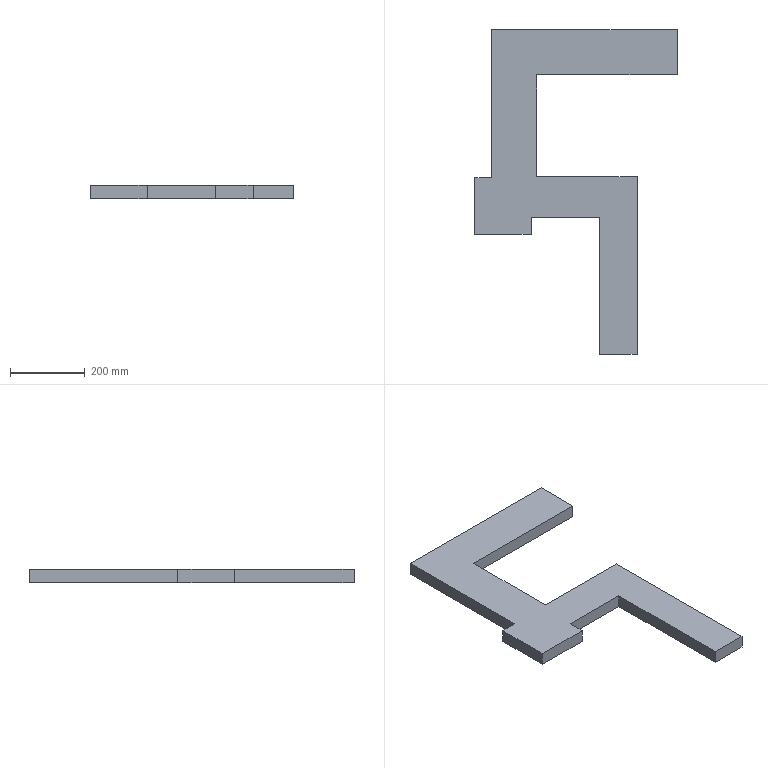Part | SolidWorks | features Extrusion 1 | 1 solid | 16 faces | box 540 x 865 x 35 mm | volume 6369754 mm3 | plane 16
STEP:
#1=CARTESIAN_POINT('',(0.,-120.,0.));
#2=VERTEX_POINT('',#1);
#3=CARTESIAN_POINT('',(0.,0.,0.));
#4=VERTEX_POINT('',#3);
#5=CARTESIAN_POINT('',(0.,0.,0.));
#6=DIRECTION('',(0.,1.,0.));
#7=VECTOR('',#6,1000.);
#8=LINE('',#5,#7);
#9=EDGE_CURVE('',#2,#4,#8,.T.);
#10=ORIENTED_EDGE('',*,*,#9,.T.);
#11=CARTESIAN_POINT('',(0.,0.,35.));
#12=VERTEX_POINT('',#11);
#13=CARTESIAN_POINT('',(0.,0.,35.));
#14=DIRECTION('',(0.,0.,-1.));
#15=VECTOR('',#14,1000.);
#16=LINE('',#13,#15);
#17=EDGE_CURVE('',#12,#4,#16,.T.);
#18=ORIENTED_EDGE('',*,*,#17,.F.);
#19=CARTESIAN_POINT('',(0.,-120.,35.));
#20=VERTEX_POINT('',#19);
#21=CARTESIAN_POINT('',(0.,0.,35.));
#22=DIRECTION('',(0.,1.,0.));
#23=VECTOR('',#22,1000.);
#24=LINE('',#21,#23);
#25=EDGE_CURVE('',#20,#12,#24,.T.);
#26=ORIENTED_EDGE('',*,*,#25,.F.);
#27=CARTESIAN_POINT('',(0.,-120.,35.));
#28=DIRECTION('',(0.,0.,-1.));
#29=VECTOR('',#28,1000.);
#30=LINE('',#27,#29);
#31=EDGE_CURVE('',#20,#2,#30,.T.);
#32=ORIENTED_EDGE('',*,*,#31,.T.);
#33=EDGE_LOOP('',(#10,#18,#26,#32));
#34=FACE_OUTER_BOUND('',#33,.T.);
#35=CARTESIAN_POINT('',(0.,0.,35.));
#36=DIRECTION('',(-1.,0.,0.));
#37=DIRECTION('',(0.,0.,1.));
#38=AXIS2_PLACEMENT_3D('',#35,#36,#37);
#39=PLANE('',#38);
#40=ADVANCED_FACE('',(#34),#39,.F.);
#41=CARTESIAN_POINT('',(-495.,0.,0.));
#42=VERTEX_POINT('',#41);
#43=CARTESIAN_POINT('',(0.,0.,0.));
#44=DIRECTION('',(-1.,0.,0.));
#45=VECTOR('',#44,1000.);
#46=LINE('',#43,#45);
#47=EDGE_CURVE('',#4,#42,#46,.T.);
#48=ORIENTED_EDGE('',*,*,#47,.T.);
#49=CARTESIAN_POINT('',(-495.,0.,35.));
#50=VERTEX_POINT('',#49);
#51=CARTESIAN_POINT('',(-495.,0.,35.));
#52=DIRECTION('',(0.,0.,-1.));
#53=VECTOR('',#52,1000.);
#54=LINE('',#51,#53);
#55=EDGE_CURVE('',#50,#42,#54,.T.);
#56=ORIENTED_EDGE('',*,*,#55,.F.);
#57=CARTESIAN_POINT('',(0.,0.,35.));
#58=DIRECTION('',(-1.,0.,0.));
#59=VECTOR('',#58,1000.);
#60=LINE('',#57,#59);
#61=EDGE_CURVE('',#12,#50,#60,.T.);
#62=ORIENTED_EDGE('',*,*,#61,.F.);
#63=ORIENTED_EDGE('',*,*,#17,.T.);
#64=EDGE_LOOP('',(#48,#56,#62,#63));
#65=FACE_OUTER_BOUND('',#64,.T.);
#66=CARTESIAN_POINT('',(0.,0.,35.));
#67=DIRECTION('',(0.,-1.,0.));
#68=DIRECTION('',(1.,0.,0.));
#69=AXIS2_PLACEMENT_3D('',#66,#67,#68);
#70=PLANE('',#69);
#71=ADVANCED_FACE('',(#65),#70,.F.);
#72=CARTESIAN_POINT('',(-495.,-395.,0.));
#73=VERTEX_POINT('',#72);
#74=CARTESIAN_POINT('',(-495.,-395.,0.));
#75=DIRECTION('',(0.,-1.,0.));
#76=VECTOR('',#75,1000.);
#77=LINE('',#74,#76);
#78=EDGE_CURVE('',#42,#73,#77,.T.);
#79=ORIENTED_EDGE('',*,*,#78,.T.);
#80=CARTESIAN_POINT('',(-495.,-395.,35.));
#81=VERTEX_POINT('',#80);
#82=CARTESIAN_POINT('',(-495.,-395.,35.));
#83=DIRECTION('',(0.,0.,-1.));
#84=VECTOR('',#83,1000.);
#85=LINE('',#82,#84);
#86=EDGE_CURVE('',#81,#73,#85,.T.);
#87=ORIENTED_EDGE('',*,*,#86,.F.);
#88=CARTESIAN_POINT('',(-495.,-395.,35.));
#89=DIRECTION('',(0.,-1.,0.));
#90=VECTOR('',#89,1000.);
#91=LINE('',#88,#90);
#92=EDGE_CURVE('',#50,#81,#91,.T.);
#93=ORIENTED_EDGE('',*,*,#92,.F.);
#94=ORIENTED_EDGE('',*,*,#55,.T.);
#95=EDGE_LOOP('',(#79,#87,#93,#94));
#96=FACE_OUTER_BOUND('',#95,.T.);
#97=CARTESIAN_POINT('',(-495.,-395.,35.));
#98=DIRECTION('',(1.,0.,0.));
#99=DIRECTION('',(0.,0.,-1.));
#100=AXIS2_PLACEMENT_3D('',#97,#98,#99);
#101=PLANE('',#100);
#102=ADVANCED_FACE('',(#96),#101,.F.);
#103=CARTESIAN_POINT('',(-540.,-395.,0.));
#104=VERTEX_POINT('',#103);
#105=CARTESIAN_POINT('',(-495.,-395.,0.));
#106=DIRECTION('',(-1.,0.,0.));
#107=VECTOR('',#106,1000.);
#108=LINE('',#105,#107);
#109=EDGE_CURVE('',#73,#104,#108,.T.);
#110=ORIENTED_EDGE('',*,*,#109,.T.);
#111=CARTESIAN_POINT('',(-540.,-395.,35.));
#112=VERTEX_POINT('',#111);
#113=CARTESIAN_POINT('',(-540.,-395.,35.));
#114=DIRECTION('',(0.,0.,-1.));
#115=VECTOR('',#114,1000.);
#116=LINE('',#113,#115);
#117=EDGE_CURVE('',#112,#104,#116,.T.);
#118=ORIENTED_EDGE('',*,*,#117,.F.);
#119=CARTESIAN_POINT('',(-495.,-395.,35.));
#120=DIRECTION('',(-1.,0.,0.));
#121=VECTOR('',#120,1000.);
#122=LINE('',#119,#121);
#123=EDGE_CURVE('',#81,#112,#122,.T.);
#124=ORIENTED_EDGE('',*,*,#123,.F.);
#125=ORIENTED_EDGE('',*,*,#86,.T.);
#126=EDGE_LOOP('',(#110,#118,#124,#125));
#127=FACE_OUTER_BOUND('',#126,.T.);
#128=CARTESIAN_POINT('',(-495.,-395.,35.));
#129=DIRECTION('',(0.,-1.,0.));
#130=DIRECTION('',(1.,0.,0.));
#131=AXIS2_PLACEMENT_3D('',#128,#129,#130);
#132=PLANE('',#131);
#133=ADVANCED_FACE('',(#127),#132,.F.);
#134=CARTESIAN_POINT('',(-540.,-545.,0.));
#135=VERTEX_POINT('',#134);
#136=CARTESIAN_POINT('',(-540.,-395.,0.));
#137=DIRECTION('',(0.,-1.,0.));
#138=VECTOR('',#137,1000.);
#139=LINE('',#136,#138);
#140=EDGE_CURVE('',#104,#135,#139,.T.);
#141=ORIENTED_EDGE('',*,*,#140,.T.);
#142=CARTESIAN_POINT('',(-540.,-545.,35.));
#143=VERTEX_POINT('',#142);
#144=CARTESIAN_POINT('',(-540.,-545.,35.));
#145=DIRECTION('',(0.,0.,-1.));
#146=VECTOR('',#145,1000.);
#147=LINE('',#144,#146);
#148=EDGE_CURVE('',#143,#135,#147,.T.);
#149=ORIENTED_EDGE('',*,*,#148,.F.);
#150=CARTESIAN_POINT('',(-540.,-395.,35.));
#151=DIRECTION('',(0.,-1.,0.));
#152=VECTOR('',#151,1000.);
#153=LINE('',#150,#152);
#154=EDGE_CURVE('',#112,#143,#153,.T.);
#155=ORIENTED_EDGE('',*,*,#154,.F.);
#156=ORIENTED_EDGE('',*,*,#117,.T.);
#157=EDGE_LOOP('',(#141,#149,#155,#156));
#158=FACE_OUTER_BOUND('',#157,.T.);
#159=CARTESIAN_POINT('',(-540.,-395.,35.));
#160=DIRECTION('',(1.,0.,0.));
#161=DIRECTION('',(0.,1.,0.));
#162=AXIS2_PLACEMENT_3D('',#159,#160,#161);
#163=PLANE('',#162);
#164=ADVANCED_FACE('',(#158),#163,.F.);
#165=CARTESIAN_POINT('',(-390.,-545.,0.));
#166=VERTEX_POINT('',#165);
#167=CARTESIAN_POINT('',(-540.,-545.,0.));
#168=DIRECTION('',(1.,0.,0.));
#169=VECTOR('',#168,1000.);
#170=LINE('',#167,#169);
#171=EDGE_CURVE('',#135,#166,#170,.T.);
#172=ORIENTED_EDGE('',*,*,#171,.T.);
#173=CARTESIAN_POINT('',(-390.,-545.,35.));
#174=VERTEX_POINT('',#173);
#175=CARTESIAN_POINT('',(-390.,-545.,35.));
#176=DIRECTION('',(0.,0.,-1.));
#177=VECTOR('',#176,1000.);
#178=LINE('',#175,#177);
#179=EDGE_CURVE('',#174,#166,#178,.T.);
#180=ORIENTED_EDGE('',*,*,#179,.F.);
#181=CARTESIAN_POINT('',(-540.,-545.,35.));
#182=DIRECTION('',(1.,0.,0.));
#183=VECTOR('',#182,1000.);
#184=LINE('',#181,#183);
#185=EDGE_CURVE('',#143,#174,#184,.T.);
#186=ORIENTED_EDGE('',*,*,#185,.F.);
#187=ORIENTED_EDGE('',*,*,#148,.T.);
#188=EDGE_LOOP('',(#172,#180,#186,#187));
#189=FACE_OUTER_BOUND('',#188,.T.);
#190=CARTESIAN_POINT('',(-540.,-545.,35.));
#191=DIRECTION('',(0.,1.,0.));
#192=DIRECTION('',(-1.,0.,0.));
#193=AXIS2_PLACEMENT_3D('',#190,#191,#192);
#194=PLANE('',#193);
#195=ADVANCED_FACE('',(#189),#194,.F.);
#196=CARTESIAN_POINT('',(-390.,-500.,0.));
#197=VERTEX_POINT('',#196);
#198=CARTESIAN_POINT('',(-390.,-545.,0.));
#199=DIRECTION('',(0.,1.,0.));
#200=VECTOR('',#199,1000.);
#201=LINE('',#198,#200);
#202=EDGE_CURVE('',#166,#197,#201,.T.);
#203=ORIENTED_EDGE('',*,*,#202,.T.);
#204=CARTESIAN_POINT('',(-390.,-500.,35.));
#205=VERTEX_POINT('',#204);
#206=CARTESIAN_POINT('',(-390.,-500.,35.));
#207=DIRECTION('',(0.,0.,-1.));
#208=VECTOR('',#207,1000.);
#209=LINE('',#206,#208);
#210=EDGE_CURVE('',#205,#197,#209,.T.);
#211=ORIENTED_EDGE('',*,*,#210,.F.);
#212=CARTESIAN_POINT('',(-390.,-545.,35.));
#213=DIRECTION('',(0.,1.,0.));
#214=VECTOR('',#213,1000.);
#215=LINE('',#212,#214);
#216=EDGE_CURVE('',#174,#205,#215,.T.);
#217=ORIENTED_EDGE('',*,*,#216,.F.);
#218=ORIENTED_EDGE('',*,*,#179,.T.);
#219=EDGE_LOOP('',(#203,#211,#217,#218));
#220=FACE_OUTER_BOUND('',#219,.T.);
#221=CARTESIAN_POINT('',(-390.,-545.,35.));
#222=DIRECTION('',(-1.,0.,0.));
#223=DIRECTION('',(0.,0.,1.));
#224=AXIS2_PLACEMENT_3D('',#221,#222,#223);
#225=PLANE('',#224);
#226=ADVANCED_FACE('',(#220),#225,.F.);
#227=CARTESIAN_POINT('',(-207.022,-500.,0.));
#228=VERTEX_POINT('',#227);
#229=CARTESIAN_POINT('',(-390.,-500.,0.));
#230=DIRECTION('',(1.,0.,0.));
#231=VECTOR('',#230,1000.);
#232=LINE('',#229,#231);
#233=EDGE_CURVE('',#197,#228,#232,.T.);
#234=ORIENTED_EDGE('',*,*,#233,.T.);
#235=CARTESIAN_POINT('',(-207.022,-500.,35.));
#236=VERTEX_POINT('',#235);
#237=CARTESIAN_POINT('',(-207.022,-500.,35.));
#238=DIRECTION('',(0.,0.,-1.));
#239=VECTOR('',#238,1000.);
#240=LINE('',#237,#239);
#241=EDGE_CURVE('',#236,#228,#240,.T.);
#242=ORIENTED_EDGE('',*,*,#241,.F.);
#243=CARTESIAN_POINT('',(-390.,-500.,35.));
#244=DIRECTION('',(1.,0.,0.));
#245=VECTOR('',#244,1000.);
#246=LINE('',#243,#245);
#247=EDGE_CURVE('',#205,#236,#246,.T.);
#248=ORIENTED_EDGE('',*,*,#247,.F.);
#249=ORIENTED_EDGE('',*,*,#210,.T.);
#250=EDGE_LOOP('',(#234,#242,#248,#249));
#251=FACE_OUTER_BOUND('',#250,.T.);
#252=CARTESIAN_POINT('',(-390.,-500.,35.));
#253=DIRECTION('',(0.,1.,0.));
#254=DIRECTION('',(-1.,0.,0.));
#255=AXIS2_PLACEMENT_3D('',#252,#253,#254);
#256=PLANE('',#255);
#257=ADVANCED_FACE('',(#251),#256,.F.);
#258=CARTESIAN_POINT('',(-207.022,-865.,0.));
#259=VERTEX_POINT('',#258);
#260=CARTESIAN_POINT('',(-207.022,-500.,0.));
#261=DIRECTION('',(0.,-1.,0.));
#262=VECTOR('',#261,1000.);
#263=LINE('',#260,#262);
#264=EDGE_CURVE('',#228,#259,#263,.T.);
#265=ORIENTED_EDGE('',*,*,#264,.T.);
#266=CARTESIAN_POINT('',(-207.022,-865.,35.));
#267=VERTEX_POINT('',#266);
#268=CARTESIAN_POINT('',(-207.022,-865.,35.));
#269=DIRECTION('',(0.,0.,-1.));
#270=VECTOR('',#269,1000.);
#271=LINE('',#268,#270);
#272=EDGE_CURVE('',#267,#259,#271,.T.);
#273=ORIENTED_EDGE('',*,*,#272,.F.);
#274=CARTESIAN_POINT('',(-207.022,-500.,35.));
#275=DIRECTION('',(0.,-1.,0.));
#276=VECTOR('',#275,1000.);
#277=LINE('',#274,#276);
#278=EDGE_CURVE('',#236,#267,#277,.T.);
#279=ORIENTED_EDGE('',*,*,#278,.F.);
#280=ORIENTED_EDGE('',*,*,#241,.T.);
#281=EDGE_LOOP('',(#265,#273,#279,#280));
#282=FACE_OUTER_BOUND('',#281,.T.);
#283=CARTESIAN_POINT('',(-207.022,-500.,35.));
#284=DIRECTION('',(1.,0.,0.));
#285=DIRECTION('',(0.,0.,-1.));
#286=AXIS2_PLACEMENT_3D('',#283,#284,#285);
#287=PLANE('',#286);
#288=ADVANCED_FACE('',(#282),#287,.F.);
#289=CARTESIAN_POINT('',(-107.022,-865.,0.));
#290=VERTEX_POINT('',#289);
#291=CARTESIAN_POINT('',(-207.022,-865.,0.));
#292=DIRECTION('',(1.,0.,0.));
#293=VECTOR('',#292,1000.);
#294=LINE('',#291,#293);
#295=EDGE_CURVE('',#259,#290,#294,.T.);
#296=ORIENTED_EDGE('',*,*,#295,.T.);
#297=CARTESIAN_POINT('',(-107.022,-865.,35.));
#298=VERTEX_POINT('',#297);
#299=CARTESIAN_POINT('',(-107.022,-865.,35.));
#300=DIRECTION('',(0.,0.,-1.));
#301=VECTOR('',#300,1000.);
#302=LINE('',#299,#301);
#303=EDGE_CURVE('',#298,#290,#302,.T.);
#304=ORIENTED_EDGE('',*,*,#303,.F.);
#305=CARTESIAN_POINT('',(-207.022,-865.,35.));
#306=DIRECTION('',(1.,0.,0.));
#307=VECTOR('',#306,1000.);
#308=LINE('',#305,#307);
#309=EDGE_CURVE('',#267,#298,#308,.T.);
#310=ORIENTED_EDGE('',*,*,#309,.F.);
#311=ORIENTED_EDGE('',*,*,#272,.T.);
#312=EDGE_LOOP('',(#296,#304,#310,#311));
#313=FACE_OUTER_BOUND('',#312,.T.);
#314=CARTESIAN_POINT('',(-207.022,-865.,35.));
#315=DIRECTION('',(0.,1.,0.));
#316=DIRECTION('',(0.,0.,1.));
#317=AXIS2_PLACEMENT_3D('',#314,#315,#316);
#318=PLANE('',#317);
#319=ADVANCED_FACE('',(#313),#318,.F.);
#320=CARTESIAN_POINT('',(-107.022,-391.715,0.));
#321=VERTEX_POINT('',#320);
#322=CARTESIAN_POINT('',(-107.022,-865.,0.));
#323=DIRECTION('',(0.,1.,0.));
#324=VECTOR('',#323,1000.);
#325=LINE('',#322,#324);
#326=EDGE_CURVE('',#290,#321,#325,.T.);
#327=ORIENTED_EDGE('',*,*,#326,.T.);
#328=CARTESIAN_POINT('',(-107.022,-391.715,35.));
#329=VERTEX_POINT('',#328);
#330=CARTESIAN_POINT('',(-107.022,-391.715,35.));
#331=DIRECTION('',(0.,0.,-1.));
#332=VECTOR('',#331,1000.);
#333=LINE('',#330,#332);
#334=EDGE_CURVE('',#329,#321,#333,.T.);
#335=ORIENTED_EDGE('',*,*,#334,.F.);
#336=CARTESIAN_POINT('',(-107.022,-865.,35.));
#337=DIRECTION('',(0.,1.,0.));
#338=VECTOR('',#337,1000.);
#339=LINE('',#336,#338);
#340=EDGE_CURVE('',#298,#329,#339,.T.);
#341=ORIENTED_EDGE('',*,*,#340,.F.);
#342=ORIENTED_EDGE('',*,*,#303,.T.);
#343=EDGE_LOOP('',(#327,#335,#341,#342));
#344=FACE_OUTER_BOUND('',#343,.T.);
#345=CARTESIAN_POINT('',(-107.022,-865.,35.));
#346=DIRECTION('',(-1.,0.,0.));
#347=DIRECTION('',(0.,0.,1.));
#348=AXIS2_PLACEMENT_3D('',#345,#346,#347);
#349=PLANE('',#348);
#350=ADVANCED_FACE('',(#344),#349,.F.);
#351=CARTESIAN_POINT('',(-375.,-391.715,0.));
#352=VERTEX_POINT('',#351);
#353=CARTESIAN_POINT('',(-107.022,-391.715,0.));
#354=DIRECTION('',(-1.,0.,0.));
#355=VECTOR('',#354,1000.);
#356=LINE('',#353,#355);
#357=EDGE_CURVE('',#321,#352,#356,.T.);
#358=ORIENTED_EDGE('',*,*,#357,.T.);
#359=CARTESIAN_POINT('',(-375.,-391.715,35.));
#360=VERTEX_POINT('',#359);
#361=CARTESIAN_POINT('',(-375.,-391.715,35.));
#362=DIRECTION('',(0.,0.,-1.));
#363=VECTOR('',#362,1000.);
#364=LINE('',#361,#363);
#365=EDGE_CURVE('',#360,#352,#364,.T.);
#366=ORIENTED_EDGE('',*,*,#365,.F.);
#367=CARTESIAN_POINT('',(-107.022,-391.715,35.));
#368=DIRECTION('',(-1.,0.,0.));
#369=VECTOR('',#368,1000.);
#370=LINE('',#367,#369);
#371=EDGE_CURVE('',#329,#360,#370,.T.);
#372=ORIENTED_EDGE('',*,*,#371,.F.);
#373=ORIENTED_EDGE('',*,*,#334,.T.);
#374=EDGE_LOOP('',(#358,#366,#372,#373));
#375=FACE_OUTER_BOUND('',#374,.T.);
#376=CARTESIAN_POINT('',(-107.022,-391.715,35.));
#377=DIRECTION('',(0.,-1.,0.));
#378=DIRECTION('',(1.,0.,0.));
#379=AXIS2_PLACEMENT_3D('',#376,#377,#378);
#380=PLANE('',#379);
#381=ADVANCED_FACE('',(#375),#380,.F.);
#382=CARTESIAN_POINT('',(-375.,-120.,0.));
#383=VERTEX_POINT('',#382);
#384=CARTESIAN_POINT('',(-375.,-120.,0.));
#385=DIRECTION('',(0.,1.,0.));
#386=VECTOR('',#385,1000.);
#387=LINE('',#384,#386);
#388=EDGE_CURVE('',#352,#383,#387,.T.);
#389=ORIENTED_EDGE('',*,*,#388,.T.);
#390=CARTESIAN_POINT('',(-375.,-120.,35.));
#391=VERTEX_POINT('',#390);
#392=CARTESIAN_POINT('',(-375.,-120.,35.));
#393=DIRECTION('',(0.,0.,-1.));
#394=VECTOR('',#393,1000.);
#395=LINE('',#392,#394);
#396=EDGE_CURVE('',#391,#383,#395,.T.);
#397=ORIENTED_EDGE('',*,*,#396,.F.);
#398=CARTESIAN_POINT('',(-375.,-120.,35.));
#399=DIRECTION('',(0.,1.,0.));
#400=VECTOR('',#399,1000.);
#401=LINE('',#398,#400);
#402=EDGE_CURVE('',#360,#391,#401,.T.);
#403=ORIENTED_EDGE('',*,*,#402,.F.);
#404=ORIENTED_EDGE('',*,*,#365,.T.);
#405=EDGE_LOOP('',(#389,#397,#403,#404));
#406=FACE_OUTER_BOUND('',#405,.T.);
#407=CARTESIAN_POINT('',(-375.,-120.,35.));
#408=DIRECTION('',(-1.,0.,0.));
#409=DIRECTION('',(0.,0.,1.));
#410=AXIS2_PLACEMENT_3D('',#407,#408,#409);
#411=PLANE('',#410);
#412=ADVANCED_FACE('',(#406),#411,.F.);
#413=CARTESIAN_POINT('',(0.,-120.,0.));
#414=DIRECTION('',(1.,0.,0.));
#415=VECTOR('',#414,1000.);
#416=LINE('',#413,#415);
#417=EDGE_CURVE('',#383,#2,#416,.T.);
#418=ORIENTED_EDGE('',*,*,#417,.T.);
#419=ORIENTED_EDGE('',*,*,#31,.F.);
#420=CARTESIAN_POINT('',(0.,-120.,35.));
#421=DIRECTION('',(1.,0.,0.));
#422=VECTOR('',#421,1000.);
#423=LINE('',#420,#422);
#424=EDGE_CURVE('',#391,#20,#423,.T.);
#425=ORIENTED_EDGE('',*,*,#424,.F.);
#426=ORIENTED_EDGE('',*,*,#396,.T.);
#427=EDGE_LOOP('',(#418,#419,#425,#426));
#428=FACE_OUTER_BOUND('',#427,.T.);
#429=CARTESIAN_POINT('',(0.,-120.,35.));
#430=DIRECTION('',(0.,1.,0.));
#431=DIRECTION('',(-1.,0.,0.));
#432=AXIS2_PLACEMENT_3D('',#429,#430,#431);
#433=PLANE('',#432);
#434=ADVANCED_FACE('',(#428),#433,.F.);
#435=ORIENTED_EDGE('',*,*,#25,.T.);
#436=ORIENTED_EDGE('',*,*,#61,.T.);
#437=ORIENTED_EDGE('',*,*,#92,.T.);
#438=ORIENTED_EDGE('',*,*,#123,.T.);
#439=ORIENTED_EDGE('',*,*,#154,.T.);
#440=ORIENTED_EDGE('',*,*,#185,.T.);
#441=ORIENTED_EDGE('',*,*,#216,.T.);
#442=ORIENTED_EDGE('',*,*,#247,.T.);
#443=ORIENTED_EDGE('',*,*,#278,.T.);
#444=ORIENTED_EDGE('',*,*,#309,.T.);
#445=ORIENTED_EDGE('',*,*,#340,.T.);
#446=ORIENTED_EDGE('',*,*,#371,.T.);
#447=ORIENTED_EDGE('',*,*,#402,.T.);
#448=ORIENTED_EDGE('',*,*,#424,.T.);
#449=EDGE_LOOP('',(#435,#436,#437,#438,#439,#440,#441,#442,#443,#444,#445,#446,#447,#448));
#450=FACE_OUTER_BOUND('',#449,.T.);
#451=CARTESIAN_POINT('',(0.,0.,35.));
#452=DIRECTION('',(0.,0.,-1.));
#453=DIRECTION('',(-1.,0.,0.));
#454=AXIS2_PLACEMENT_3D('',#451,#452,#453);
#455=PLANE('',#454);
#456=ADVANCED_FACE('',(#450),#455,.F.);
#457=ORIENTED_EDGE('',*,*,#9,.F.);
#458=ORIENTED_EDGE('',*,*,#417,.F.);
#459=ORIENTED_EDGE('',*,*,#388,.F.);
#460=ORIENTED_EDGE('',*,*,#357,.F.);
#461=ORIENTED_EDGE('',*,*,#326,.F.);
#462=ORIENTED_EDGE('',*,*,#295,.F.);
#463=ORIENTED_EDGE('',*,*,#264,.F.);
#464=ORIENTED_EDGE('',*,*,#233,.F.);
#465=ORIENTED_EDGE('',*,*,#202,.F.);
#466=ORIENTED_EDGE('',*,*,#171,.F.);
#467=ORIENTED_EDGE('',*,*,#140,.F.);
#468=ORIENTED_EDGE('',*,*,#109,.F.);
#469=ORIENTED_EDGE('',*,*,#78,.F.);
#470=ORIENTED_EDGE('',*,*,#47,.F.);
#471=EDGE_LOOP('',(#457,#458,#459,#460,#461,#462,#463,#464,#465,#466,#467,#468,#469,#470));
#472=FACE_OUTER_BOUND('',#471,.T.);
#473=CARTESIAN_POINT('',(0.,0.,0.));
#474=DIRECTION('',(0.,0.,-1.));
#475=DIRECTION('',(-1.,0.,0.));
#476=AXIS2_PLACEMENT_3D('',#473,#474,#475);
#477=PLANE('',#476);
#478=ADVANCED_FACE('',(#472),#477,.T.);
#479=CLOSED_SHELL('',(#40,#71,#102,#133,#164,#195,#226,#257,#288,#319,#350,#381,#412,#434,#456,#478));
#480=MANIFOLD_SOLID_BREP('',#479);
#481=CARTESIAN_POINT('',(0.,0.,0.));
#482=DIRECTION('',(0.,0.,1.));
#483=DIRECTION('',(1.,0.,0.));
#484=AXIS2_PLACEMENT_3D('',#481,#482,#483);
#485=(LENGTH_UNIT()NAMED_UNIT(*)SI_UNIT(.MILLI.,.METRE.));
#486=UNCERTAINTY_MEASURE_WITH_UNIT(LENGTH_MEASURE(0.00001),#485,'','');
#487=(NAMED_UNIT(*)PLANE_ANGLE_UNIT()SI_UNIT($,.RADIAN.));
#488=(NAMED_UNIT(*)SI_UNIT($,.STERADIAN.)SOLID_ANGLE_UNIT());
#489=(GEOMETRIC_REPRESENTATION_CONTEXT(3)GLOBAL_UNCERTAINTY_ASSIGNED_CONTEXT((#486))GLOBAL_UNIT_ASSIGNED_CONTEXT((#485,#487,#488))REPRESENTATION_CONTEXT('',''));
#490=ADVANCED_BREP_SHAPE_REPRESENTATION('',(#480,#484),#489);